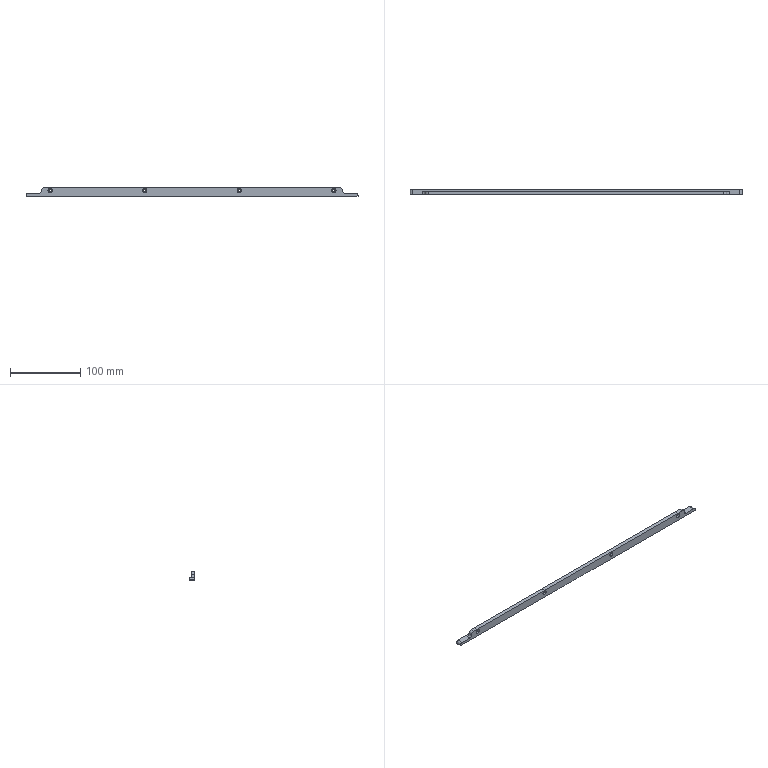CAM job | NX | 3+2 milling, drilling | part box 474 x 8.3 x 12 mm | stock box 479 x 10 x 17 mm
Tools:
number,name,description,diameter,corner_radius,flute_length,length,flutes
4,D4,平底铣刀-粗,4.0,0.0,25.0,75.0,2
9,D10,平底铣刀-粗,10.0,0.0,35.0,75.0,2
11,D4-J,平底铣刀-精,4.0,0.0,50.0,75.0,2
7,D6-J,平底铣刀-精,6.0,0.0,25.0,75.0,2
10,D10-J,平底铣刀-精,10.0,0.0,35.0,75.0,2
1,D80R0.8飞刀,圆鼻刀-粗,80.0,0.8,50.0,75.0,2
17,D6R0.5-J,圆鼻刀-精,6.0,0.5,50.0,75.0,2
1,D80R0.8飞刀-J,圆鼻刀-精,80.0,0.8,50.0,75.0,2
2,D6倒角刀,倒角刀,6.0,0.0,3.0,25.0,2
13,ZT3.4,钻头,3.4,0.0,35.0,50.0,2
Operations:
program,operation,operation_type,tool,method,geometry_group,spindle_rpm,surface_speed,feed_per_tooth,feed_cut,feed_plunge,cut_length_mm,path_length_mm,cut_time_min,machine_time_min
B,FLOORFACEONECUTROUGH_COPY,VolumeBased25DMillingOperation,D80R0.8飞刀,LAYERROUGH-DEPTHK-STEPG,W-B,2800.0,703.696,0.5357,3000.0,100.0,2326.425,4093.619,0.7755,0.9522
B,FLOORFACEONECUTFINISH_COPY,VolumeBased25DMillingOperation,D80R0.8飞刀-J,SIDEFINISH-DEPTHK-STEPG,W-B,4000.0,1005.28,0.125,1000.0,100.0,581.41,617.41,0.5814,0.585
B,FLOORLAYERROUGHMID_COPY,VolumeBased25DMillingOperation,D10,LAYERROUGH-DEPTHK-STEPG,W-B,8000.0,251.32,0.25,4000.0,100.0,4466.614,4513.525,1.117,1.121
B,ZLEVELFINISHRECIPSLOPE_COPY,ZLevelMilling,D6R0.5-J,ZLEVELSLOPE-DEPTHK-STEPG,W-B,7000.0,131.947,0.2857,4000.0,100.0,699.569,1227.015,0.1749,0.2276
B,DRILLCHAMFER_1,Operation,D6倒角刀,METHOD,W-B,8000.0,150.796,0.0625,1000.0,0.0,20.0,500.7,0.02,0.0681
B,PLANARDEBURR6X45L_COPY,SurfaceContour,D6倒角刀,SLOPE_CHAMFER-DEPTH0-STEPG,W-B,6500.0,122.519,0.1154,1500.0,100.0,1430.791,2030.939,0.9539,1.014
B,FLOORSIDEFINISHMID-SELFLOOR_COPY,VolumeBased25DMillingOperation,D10-J,SIDEFINISH-DEPTHK-STEPG,W-B,8000.0,251.32,0.0625,1000.0,100.0,448.572,476.172,0.4486,0.4513
A,TOPFACEROUGH,FaceMilling,D80R0.8飞刀,LAYERROUGH-DEPTHK-STEPG,W-A,4000.0,1005.31,0.375,3000.0,100.0,568.0,603.8,0.1893,0.1929
A,TOPFACE,FaceMilling,D80R0.8飞刀,SIDEFINISH-DEPTHK-STEPG,W-A,4000.0,1005.31,0.125,1000.0,100.0,568.0,604.0,0.568,0.5716
A,PROFILEROUGH_2,VolumeBased25DMillingOperation,D10,METHOD,W-A,8000.0,251.327,0.3125,5000.0,80.0,11926.931,11973.73,2.385,2.39
A,CSINKSPOT-DEPTH0.8,Operation,D6倒角刀,NONE,W-A,8000.0,150.796,0.0312,500.0,90.0,7.2,462.411,0.0144,0.0599
A,CSINK-DRILL0SEG,Operation,ZT3.4,NONE,W-A,2800.0,29.908,0.0179,100.0,90.0,36.086,520.183,0.3609,0.4093
A,CYLROUGHD4_1,CylinderMilling,D4,NONE,W-A,8000.0,100.531,0.075,1200.0,100.0,419.412,996.012,0.3495,0.4072
A,CYLFINISHD4_1,CylinderMilling,D4-J,FINISH-STEPDEPTHOFF,W-A,8000.0,100.531,0.0312,500.0,100.0,75.825,652.424,0.1516,0.2093
A,PROFILESIDE,ZLevelMilling,D6-J,METHOD,W-A,9000.0,84.823,0.1389,2500.0,80.0,441.612,972.51,0.177,0.2301
A,BODYONLY,SurfaceContour,D6倒角刀,METHOD,W-A,8000.0,150.796,0.1875,3000.0,100.0,979.872,1015.673,0.3266,0.3302
A,MILLCHAMFER_1,PlanarMilling,D6倒角刀,NONE,W-A,8000.0,150.796,0.0312,500.0,100.0,117.022,669.253,0.234,0.2893
A,PROFILESEMI_2,VolumeBased25DMillingOperation,D6-J,METHOD,W-A,8000.0,251.327,0.0625,1000.0,100.0,986.323,1041.923,0.9863,0.9919